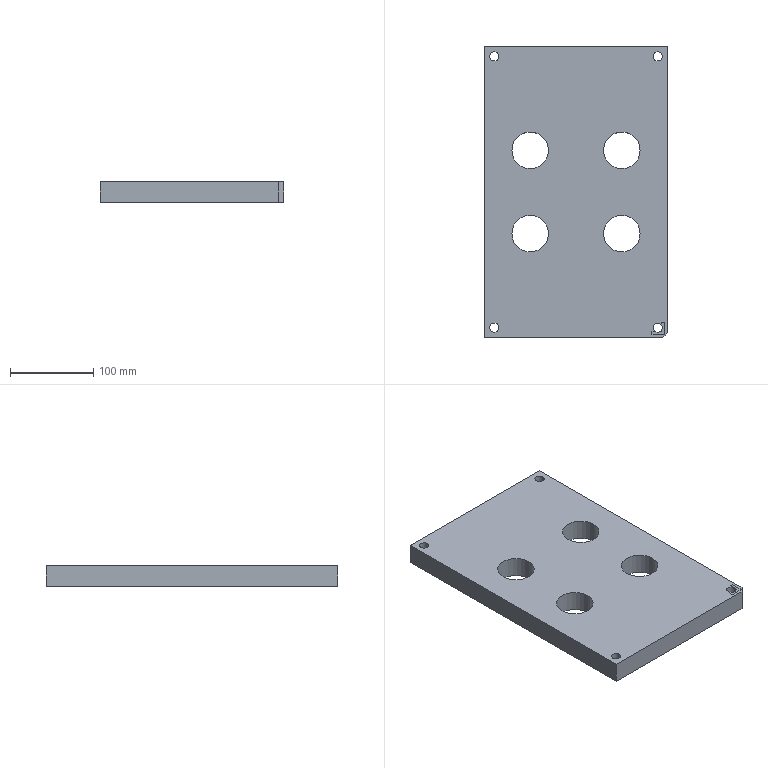Part | NX | features DZDB 2 | 1 solid | 33 faces | box 220 x 350 x 25 mm | volume 1756097 mm3 | plane 21 | cylinder 12 | commonest cylinder face diameters 11 x4 18 x4 44 x4
STEP:
#1=CARTESIAN_POINT('',(-77.,50.,-235.5));
#2=VERTEX_POINT('',#1);
#3=CARTESIAN_POINT('',(-55.,50.,-235.5));
#4=DIRECTION('',(0.,0.,-1.));
#5=DIRECTION('',(-1.,0.,0.));
#6=AXIS2_PLACEMENT_3D('',#3,#4,#5);
#7=CIRCLE('',#6,22.);
#8=EDGE_CURVE('',#2,#2,#7,.T.);
#9=ORIENTED_EDGE('',*,*,#8,.F.);
#10=EDGE_LOOP('',(#9));
#11=FACE_BOUND('',#10,.T.);
#12=CARTESIAN_POINT('',(33.,50.,-235.5));
#13=VERTEX_POINT('',#12);
#14=CARTESIAN_POINT('',(55.,50.,-235.5));
#15=DIRECTION('',(0.,0.,-1.));
#16=DIRECTION('',(-1.,0.,0.));
#17=AXIS2_PLACEMENT_3D('',#14,#15,#16);
#18=CIRCLE('',#17,22.);
#19=EDGE_CURVE('',#13,#13,#18,.T.);
#20=ORIENTED_EDGE('',*,*,#19,.F.);
#21=EDGE_LOOP('',(#20));
#22=FACE_BOUND('',#21,.T.);
#23=CARTESIAN_POINT('',(33.,-50.,-235.5));
#24=VERTEX_POINT('',#23);
#25=CARTESIAN_POINT('',(55.,-50.,-235.5));
#26=DIRECTION('',(0.,0.,-1.));
#27=DIRECTION('',(-1.,0.,0.));
#28=AXIS2_PLACEMENT_3D('',#25,#26,#27);
#29=CIRCLE('',#28,22.);
#30=EDGE_CURVE('',#24,#24,#29,.T.);
#31=ORIENTED_EDGE('',*,*,#30,.F.);
#32=EDGE_LOOP('',(#31));
#33=FACE_BOUND('',#32,.T.);
#34=CARTESIAN_POINT('',(-77.,-50.,-235.5));
#35=VERTEX_POINT('',#34);
#36=CARTESIAN_POINT('',(-55.,-50.,-235.5));
#37=DIRECTION('',(0.,0.,-1.));
#38=DIRECTION('',(-1.,0.,0.));
#39=AXIS2_PLACEMENT_3D('',#36,#37,#38);
#40=CIRCLE('',#39,22.);
#41=EDGE_CURVE('',#35,#35,#40,.T.);
#42=ORIENTED_EDGE('',*,*,#41,.F.);
#43=EDGE_LOOP('',(#42));
#44=FACE_BOUND('',#43,.T.);
#45=CARTESIAN_POINT('',(-107.,-163.,-235.5));
#46=VERTEX_POINT('',#45);
#47=CARTESIAN_POINT('',(-98.,-163.,-235.5));
#48=DIRECTION('',(0.,0.,1.));
#49=DIRECTION('',(-1.,0.,0.));
#50=AXIS2_PLACEMENT_3D('',#47,#48,#49);
#51=CIRCLE('',#50,9.);
#52=EDGE_CURVE('',#46,#46,#51,.T.);
#53=ORIENTED_EDGE('',*,*,#52,.T.);
#54=EDGE_LOOP('',(#53));
#55=FACE_BOUND('',#54,.T.);
#56=CARTESIAN_POINT('',(107.,163.,-235.5));
#57=VERTEX_POINT('',#56);
#58=CARTESIAN_POINT('',(98.,163.,-235.5));
#59=DIRECTION('',(0.,0.,1.));
#60=DIRECTION('',(1.,0.,0.));
#61=AXIS2_PLACEMENT_3D('',#58,#59,#60);
#62=CIRCLE('',#61,9.);
#63=EDGE_CURVE('',#57,#57,#62,.T.);
#64=ORIENTED_EDGE('',*,*,#63,.T.);
#65=EDGE_LOOP('',(#64));
#66=FACE_BOUND('',#65,.T.);
#67=CARTESIAN_POINT('',(110.,-169.,-235.5));
#68=VERTEX_POINT('',#67);
#69=CARTESIAN_POINT('',(110.,175.,-235.5));
#70=VERTEX_POINT('',#69);
#71=CARTESIAN_POINT('',(110.,0.,-235.5));
#72=DIRECTION('',(0.,1.,0.));
#73=VECTOR('',#72,1000.);
#74=LINE('',#71,#73);
#75=EDGE_CURVE('',#68,#70,#74,.T.);
#76=ORIENTED_EDGE('',*,*,#75,.F.);
#77=CARTESIAN_POINT('',(104.,-175.,-235.5));
#78=VERTEX_POINT('',#77);
#79=CARTESIAN_POINT('',(139.5,-139.5,-235.5));
#80=DIRECTION('',(0.7071,0.7071,0.));
#81=VECTOR('',#80,1000.);
#82=LINE('',#79,#81);
#83=EDGE_CURVE('',#68,#78,#82,.F.);
#84=ORIENTED_EDGE('',*,*,#83,.T.);
#85=CARTESIAN_POINT('',(-110.,-175.,-235.5));
#86=VERTEX_POINT('',#85);
#87=CARTESIAN_POINT('',(0.,-175.,-235.5));
#88=DIRECTION('',(1.,0.,0.));
#89=VECTOR('',#88,1000.);
#90=LINE('',#87,#89);
#91=EDGE_CURVE('',#86,#78,#90,.T.);
#92=ORIENTED_EDGE('',*,*,#91,.F.);
#93=CARTESIAN_POINT('',(-110.,175.,-235.5));
#94=VERTEX_POINT('',#93);
#95=CARTESIAN_POINT('',(-110.,0.,-235.5));
#96=DIRECTION('',(0.,-1.,0.));
#97=VECTOR('',#96,1000.);
#98=LINE('',#95,#97);
#99=EDGE_CURVE('',#94,#86,#98,.T.);
#100=ORIENTED_EDGE('',*,*,#99,.F.);
#101=CARTESIAN_POINT('',(0.,175.,-235.5));
#102=DIRECTION('',(-1.,0.,0.));
#103=VECTOR('',#102,1000.);
#104=LINE('',#101,#103);
#105=EDGE_CURVE('',#70,#94,#104,.T.);
#106=ORIENTED_EDGE('',*,*,#105,.F.);
#107=EDGE_LOOP('',(#76,#84,#92,#100,#106));
#108=FACE_BOUND('',#107,.T.);
#109=CARTESIAN_POINT('',(107.,-163.,-235.5));
#110=VERTEX_POINT('',#109);
#111=CARTESIAN_POINT('',(98.,-163.,-235.5));
#112=DIRECTION('',(0.,0.,1.));
#113=DIRECTION('',(1.,0.,0.));
#114=AXIS2_PLACEMENT_3D('',#111,#112,#113);
#115=CIRCLE('',#114,9.);
#116=EDGE_CURVE('',#110,#110,#115,.T.);
#117=ORIENTED_EDGE('',*,*,#116,.T.);
#118=EDGE_LOOP('',(#117));
#119=FACE_BOUND('',#118,.T.);
#120=CARTESIAN_POINT('',(-89.,163.,-235.5));
#121=VERTEX_POINT('',#120);
#122=CARTESIAN_POINT('',(-98.,163.,-235.5));
#123=DIRECTION('',(0.,0.,1.));
#124=DIRECTION('',(1.,0.,0.));
#125=AXIS2_PLACEMENT_3D('',#122,#123,#124);
#126=CIRCLE('',#125,9.);
#127=EDGE_CURVE('',#121,#121,#126,.T.);
#128=ORIENTED_EDGE('',*,*,#127,.T.);
#129=EDGE_LOOP('',(#128));
#130=FACE_BOUND('',#129,.T.);
#131=CARTESIAN_POINT('',(0.,0.,-235.5));
#132=DIRECTION('',(0.,0.,-1.));
#133=DIRECTION('',(-1.,0.,0.));
#134=AXIS2_PLACEMENT_3D('',#131,#132,#133);
#135=PLANE('',#134);
#136=ADVANCED_FACE('',(#11,#22,#33,#44,#55,#66,#108,#119,#130),#135,.T.);
#137=CARTESIAN_POINT('',(-33.,50.,-210.5));
#138=VERTEX_POINT('',#137);
#139=CARTESIAN_POINT('',(-55.,50.,-210.5));
#140=DIRECTION('',(0.,0.,1.));
#141=DIRECTION('',(1.,0.,0.));
#142=AXIS2_PLACEMENT_3D('',#139,#140,#141);
#143=CIRCLE('',#142,22.);
#144=EDGE_CURVE('',#138,#138,#143,.T.);
#145=ORIENTED_EDGE('',*,*,#144,.F.);
#146=EDGE_LOOP('',(#145));
#147=FACE_BOUND('',#146,.T.);
#148=CARTESIAN_POINT('',(77.,50.,-210.5));
#149=VERTEX_POINT('',#148);
#150=CARTESIAN_POINT('',(55.,50.,-210.5));
#151=DIRECTION('',(0.,0.,1.));
#152=DIRECTION('',(1.,0.,0.));
#153=AXIS2_PLACEMENT_3D('',#150,#151,#152);
#154=CIRCLE('',#153,22.);
#155=EDGE_CURVE('',#149,#149,#154,.T.);
#156=ORIENTED_EDGE('',*,*,#155,.F.);
#157=EDGE_LOOP('',(#156));
#158=FACE_BOUND('',#157,.T.);
#159=CARTESIAN_POINT('',(77.,-50.,-210.5));
#160=VERTEX_POINT('',#159);
#161=CARTESIAN_POINT('',(55.,-50.,-210.5));
#162=DIRECTION('',(0.,0.,1.));
#163=DIRECTION('',(1.,0.,0.));
#164=AXIS2_PLACEMENT_3D('',#161,#162,#163);
#165=CIRCLE('',#164,22.);
#166=EDGE_CURVE('',#160,#160,#165,.T.);
#167=ORIENTED_EDGE('',*,*,#166,.F.);
#168=EDGE_LOOP('',(#167));
#169=FACE_BOUND('',#168,.T.);
#170=CARTESIAN_POINT('',(-33.,-50.,-210.5));
#171=VERTEX_POINT('',#170);
#172=CARTESIAN_POINT('',(-55.,-50.,-210.5));
#173=DIRECTION('',(0.,0.,1.));
#174=DIRECTION('',(1.,0.,0.));
#175=AXIS2_PLACEMENT_3D('',#172,#173,#174);
#176=CIRCLE('',#175,22.);
#177=EDGE_CURVE('',#171,#171,#176,.T.);
#178=ORIENTED_EDGE('',*,*,#177,.F.);
#179=EDGE_LOOP('',(#178));
#180=FACE_BOUND('',#179,.T.);
#181=CARTESIAN_POINT('',(-103.5,-163.,-210.5));
#182=VERTEX_POINT('',#181);
#183=CARTESIAN_POINT('',(-98.,-163.,-210.5));
#184=DIRECTION('',(0.,0.,-1.));
#185=DIRECTION('',(-1.,0.,0.));
#186=AXIS2_PLACEMENT_3D('',#183,#184,#185);
#187=CIRCLE('',#186,5.5);
#188=EDGE_CURVE('',#182,#182,#187,.T.);
#189=ORIENTED_EDGE('',*,*,#188,.T.);
#190=EDGE_LOOP('',(#189));
#191=FACE_BOUND('',#190,.T.);
#192=CARTESIAN_POINT('',(103.5,163.,-210.5));
#193=VERTEX_POINT('',#192);
#194=CARTESIAN_POINT('',(98.,163.,-210.5));
#195=DIRECTION('',(0.,0.,-1.));
#196=DIRECTION('',(1.,0.,0.));
#197=AXIS2_PLACEMENT_3D('',#194,#195,#196);
#198=CIRCLE('',#197,5.5);
#199=EDGE_CURVE('',#193,#193,#198,.T.);
#200=ORIENTED_EDGE('',*,*,#199,.T.);
#201=EDGE_LOOP('',(#200));
#202=FACE_BOUND('',#201,.T.);
#203=CARTESIAN_POINT('',(104.,-175.,-210.5));
#204=VERTEX_POINT('',#203);
#205=CARTESIAN_POINT('',(-110.,-175.,-210.5));
#206=VERTEX_POINT('',#205);
#207=CARTESIAN_POINT('',(0.,-175.,-210.5));
#208=DIRECTION('',(-1.,0.,0.));
#209=VECTOR('',#208,1000.);
#210=LINE('',#207,#209);
#211=EDGE_CURVE('',#204,#206,#210,.T.);
#212=ORIENTED_EDGE('',*,*,#211,.F.);
#213=CARTESIAN_POINT('',(110.,-169.,-210.5));
#214=VERTEX_POINT('',#213);
#215=CARTESIAN_POINT('',(139.5,-139.5,-210.5));
#216=DIRECTION('',(-0.7071,-0.7071,0.));
#217=VECTOR('',#216,1000.);
#218=LINE('',#215,#217);
#219=EDGE_CURVE('',#204,#214,#218,.F.);
#220=ORIENTED_EDGE('',*,*,#219,.T.);
#221=CARTESIAN_POINT('',(110.,175.,-210.5));
#222=VERTEX_POINT('',#221);
#223=CARTESIAN_POINT('',(110.,0.,-210.5));
#224=DIRECTION('',(0.,-1.,0.));
#225=VECTOR('',#224,1000.);
#226=LINE('',#223,#225);
#227=EDGE_CURVE('',#222,#214,#226,.T.);
#228=ORIENTED_EDGE('',*,*,#227,.F.);
#229=CARTESIAN_POINT('',(-110.,175.,-210.5));
#230=VERTEX_POINT('',#229);
#231=CARTESIAN_POINT('',(0.,175.,-210.5));
#232=DIRECTION('',(1.,0.,0.));
#233=VECTOR('',#232,1000.);
#234=LINE('',#231,#233);
#235=EDGE_CURVE('',#230,#222,#234,.T.);
#236=ORIENTED_EDGE('',*,*,#235,.F.);
#237=CARTESIAN_POINT('',(-110.,0.,-210.5));
#238=DIRECTION('',(0.,1.,0.));
#239=VECTOR('',#238,1000.);
#240=LINE('',#237,#239);
#241=EDGE_CURVE('',#206,#230,#240,.T.);
#242=ORIENTED_EDGE('',*,*,#241,.F.);
#243=EDGE_LOOP('',(#212,#220,#228,#236,#242));
#244=FACE_BOUND('',#243,.T.);
#245=CARTESIAN_POINT('',(94.838,-167.5,-210.5));
#246=VERTEX_POINT('',#245);
#247=CARTESIAN_POINT('',(91.25,-167.5,-210.5));
#248=VERTEX_POINT('',#247);
#249=CARTESIAN_POINT('',(96.875,-167.5,-210.5));
#250=DIRECTION('',(-1.,0.,0.));
#251=VECTOR('',#250,1000.);
#252=LINE('',#249,#251);
#253=EDGE_CURVE('',#246,#248,#252,.T.);
#254=ORIENTED_EDGE('',*,*,#253,.F.);
#255=CARTESIAN_POINT('',(102.5,-159.838,-210.5));
#256=VERTEX_POINT('',#255);
#257=CARTESIAN_POINT('',(98.,-163.,-210.5));
#258=DIRECTION('',(0.,0.,-1.));
#259=DIRECTION('',(1.,0.,0.));
#260=AXIS2_PLACEMENT_3D('',#257,#258,#259);
#261=CIRCLE('',#260,5.5);
#262=EDGE_CURVE('',#246,#256,#261,.T.);
#263=ORIENTED_EDGE('',*,*,#262,.T.);
#264=CARTESIAN_POINT('',(102.5,-156.25,-210.5));
#265=VERTEX_POINT('',#264);
#266=CARTESIAN_POINT('',(102.5,-161.875,-210.5));
#267=DIRECTION('',(0.,-1.,0.));
#268=VECTOR('',#267,1000.);
#269=LINE('',#266,#268);
#270=EDGE_CURVE('',#265,#256,#269,.T.);
#271=ORIENTED_EDGE('',*,*,#270,.F.);
#272=CARTESIAN_POINT('',(106.25,-156.25,-210.5));
#273=VERTEX_POINT('',#272);
#274=CARTESIAN_POINT('',(98.75,-156.25,-210.5));
#275=DIRECTION('',(1.,0.,0.));
#276=VECTOR('',#275,1000.);
#277=LINE('',#274,#276);
#278=EDGE_CURVE('',#265,#273,#277,.T.);
#279=ORIENTED_EDGE('',*,*,#278,.T.);
#280=CARTESIAN_POINT('',(106.25,-171.25,-210.5));
#281=VERTEX_POINT('',#280);
#282=CARTESIAN_POINT('',(106.25,-163.75,-210.5));
#283=DIRECTION('',(0.,-1.,0.));
#284=VECTOR('',#283,1000.);
#285=LINE('',#282,#284);
#286=EDGE_CURVE('',#273,#281,#285,.T.);
#287=ORIENTED_EDGE('',*,*,#286,.T.);
#288=CARTESIAN_POINT('',(91.25,-171.25,-210.5));
#289=VERTEX_POINT('',#288);
#290=CARTESIAN_POINT('',(98.75,-171.25,-210.5));
#291=DIRECTION('',(-1.,0.,0.));
#292=VECTOR('',#291,1000.);
#293=LINE('',#290,#292);
#294=EDGE_CURVE('',#281,#289,#293,.T.);
#295=ORIENTED_EDGE('',*,*,#294,.T.);
#296=CARTESIAN_POINT('',(91.25,-163.75,-210.5));
#297=DIRECTION('',(0.,1.,0.));
#298=VECTOR('',#297,1000.);
#299=LINE('',#296,#298);
#300=EDGE_CURVE('',#289,#248,#299,.T.);
#301=ORIENTED_EDGE('',*,*,#300,.T.);
#302=EDGE_LOOP('',(#254,#263,#271,#279,#287,#295,#301));
#303=FACE_BOUND('',#302,.T.);
#304=CARTESIAN_POINT('',(-92.5,163.,-210.5));
#305=VERTEX_POINT('',#304);
#306=CARTESIAN_POINT('',(-98.,163.,-210.5));
#307=DIRECTION('',(0.,0.,-1.));
#308=DIRECTION('',(1.,0.,0.));
#309=AXIS2_PLACEMENT_3D('',#306,#307,#308);
#310=CIRCLE('',#309,5.5);
#311=EDGE_CURVE('',#305,#305,#310,.T.);
#312=ORIENTED_EDGE('',*,*,#311,.T.);
#313=EDGE_LOOP('',(#312));
#314=FACE_BOUND('',#313,.T.);
#315=CARTESIAN_POINT('',(0.,0.,-210.5));
#316=DIRECTION('',(0.,0.,1.));
#317=DIRECTION('',(1.,0.,0.));
#318=AXIS2_PLACEMENT_3D('',#315,#316,#317);
#319=PLANE('',#318);
#320=ADVANCED_FACE('',(#147,#158,#169,#180,#191,#202,#244,#303,#314),#319,.T.);
#321=CARTESIAN_POINT('',(102.5,-166.162,-210.5));
#322=VERTEX_POINT('',#321);
#323=CARTESIAN_POINT('',(102.5,-167.5,-210.5));
#324=VERTEX_POINT('',#323);
#325=CARTESIAN_POINT('',(102.5,-161.875,-210.5));
#326=DIRECTION('',(0.,-1.,0.));
#327=VECTOR('',#326,1000.);
#328=LINE('',#325,#327);
#329=EDGE_CURVE('',#322,#324,#328,.T.);
#330=ORIENTED_EDGE('',*,*,#329,.F.);
#331=CARTESIAN_POINT('',(101.162,-167.5,-210.5));
#332=VERTEX_POINT('',#331);
#333=CARTESIAN_POINT('',(98.,-163.,-210.5));
#334=DIRECTION('',(0.,0.,-1.));
#335=DIRECTION('',(1.,0.,0.));
#336=AXIS2_PLACEMENT_3D('',#333,#334,#335);
#337=CIRCLE('',#336,5.5);
#338=EDGE_CURVE('',#322,#332,#337,.T.);
#339=ORIENTED_EDGE('',*,*,#338,.T.);
#340=CARTESIAN_POINT('',(96.875,-167.5,-210.5));
#341=DIRECTION('',(-1.,0.,0.));
#342=VECTOR('',#341,1000.);
#343=LINE('',#340,#342);
#344=EDGE_CURVE('',#324,#332,#343,.T.);
#345=ORIENTED_EDGE('',*,*,#344,.F.);
#346=EDGE_LOOP('',(#330,#339,#345));
#347=FACE_BOUND('',#346,.T.);
#348=CARTESIAN_POINT('',(0.,0.,-210.5));
#349=DIRECTION('',(0.,0.,1.));
#350=DIRECTION('',(1.,0.,0.));
#351=AXIS2_PLACEMENT_3D('',#348,#349,#350);
#352=PLANE('',#351);
#353=ADVANCED_FACE('',(#347),#352,.T.);
#354=CARTESIAN_POINT('',(101.162,-167.5,-210.6));
#355=VERTEX_POINT('',#354);
#356=CARTESIAN_POINT('',(101.162,-167.5,-235.5));
#357=DIRECTION('',(0.,0.,1.));
#358=VECTOR('',#357,1000.);
#359=LINE('',#356,#358);
#360=EDGE_CURVE('',#355,#332,#359,.T.);
#361=ORIENTED_EDGE('',*,*,#360,.F.);
#362=CARTESIAN_POINT('',(102.5,-167.5,-210.6));
#363=VERTEX_POINT('',#362);
#364=CARTESIAN_POINT('',(96.875,-167.5,-210.6));
#365=DIRECTION('',(1.,0.,0.));
#366=VECTOR('',#365,1000.);
#367=LINE('',#364,#366);
#368=EDGE_CURVE('',#363,#355,#367,.F.);
#369=ORIENTED_EDGE('',*,*,#368,.F.);
#370=CARTESIAN_POINT('',(102.5,-167.5,-210.6));
#371=DIRECTION('',(0.,0.,1.));
#372=VECTOR('',#371,1000.);
#373=LINE('',#370,#372);
#374=EDGE_CURVE('',#363,#324,#373,.T.);
#375=ORIENTED_EDGE('',*,*,#374,.T.);
#376=ORIENTED_EDGE('',*,*,#344,.T.);
#377=EDGE_LOOP('',(#361,#369,#375,#376));
#378=FACE_BOUND('',#377,.T.);
#379=CARTESIAN_POINT('',(96.875,-167.5,-210.6));
#380=DIRECTION('',(0.,-1.,0.));
#381=DIRECTION('',(0.,0.,-1.));
#382=AXIS2_PLACEMENT_3D('',#379,#380,#381);
#383=PLANE('',#382);
#384=ADVANCED_FACE('',(#378),#383,.T.);
#385=CARTESIAN_POINT('',(102.5,-159.838,-210.6));
#386=VERTEX_POINT('',#385);
#387=CARTESIAN_POINT('',(102.5,-159.838,-235.5));
#388=DIRECTION('',(0.,0.,1.));
#389=VECTOR('',#388,1000.);
#390=LINE('',#387,#389);
#391=EDGE_CURVE('',#386,#256,#390,.T.);
#392=ORIENTED_EDGE('',*,*,#391,.F.);
#393=CARTESIAN_POINT('',(102.5,-156.25,-210.6));
#394=VERTEX_POINT('',#393);
#395=CARTESIAN_POINT('',(102.5,-161.875,-210.6));
#396=DIRECTION('',(0.,1.,0.));
#397=VECTOR('',#396,1000.);
#398=LINE('',#395,#397);
#399=EDGE_CURVE('',#394,#386,#398,.F.);
#400=ORIENTED_EDGE('',*,*,#399,.F.);
#401=CARTESIAN_POINT('',(102.5,-156.25,-210.6));
#402=DIRECTION('',(0.,0.,1.));
#403=VECTOR('',#402,1000.);
#404=LINE('',#401,#403);
#405=EDGE_CURVE('',#265,#394,#404,.F.);
#406=ORIENTED_EDGE('',*,*,#405,.F.);
#407=ORIENTED_EDGE('',*,*,#270,.T.);
#408=EDGE_LOOP('',(#392,#400,#406,#407));
#409=FACE_BOUND('',#408,.T.);
#410=CARTESIAN_POINT('',(102.5,-161.875,-210.6));
#411=DIRECTION('',(1.,0.,0.));
#412=DIRECTION('',(0.,0.,-1.));
#413=AXIS2_PLACEMENT_3D('',#410,#411,#412);
#414=PLANE('',#413);
#415=ADVANCED_FACE('',(#409),#414,.T.);
#416=ORIENTED_EDGE('',*,*,#91,.T.);
#417=CARTESIAN_POINT('',(104.,-175.,-235.5));
#418=DIRECTION('',(0.,0.,1.));
#419=VECTOR('',#418,1000.);
#420=LINE('',#417,#419);
#421=EDGE_CURVE('',#78,#204,#420,.T.);
#422=ORIENTED_EDGE('',*,*,#421,.T.);
#423=ORIENTED_EDGE('',*,*,#211,.T.);
#424=CARTESIAN_POINT('',(-110.,-175.,-235.5));
#425=DIRECTION('',(0.,0.,1.));
#426=VECTOR('',#425,1000.);
#427=LINE('',#424,#426);
#428=EDGE_CURVE('',#86,#206,#427,.T.);
#429=ORIENTED_EDGE('',*,*,#428,.F.);
#430=EDGE_LOOP('',(#416,#422,#423,#429));
#431=FACE_BOUND('',#430,.T.);
#432=CARTESIAN_POINT('',(0.,-175.,-235.5));
#433=DIRECTION('',(0.,-1.,0.));
#434=DIRECTION('',(0.,0.,-1.));
#435=AXIS2_PLACEMENT_3D('',#432,#433,#434);
#436=PLANE('',#435);
#437=ADVANCED_FACE('',(#431),#436,.T.);
#438=ORIENTED_EDGE('',*,*,#428,.T.);
#439=ORIENTED_EDGE('',*,*,#241,.T.);
#440=CARTESIAN_POINT('',(-110.,175.,-235.5));
#441=DIRECTION('',(0.,0.,1.));
#442=VECTOR('',#441,1000.);
#443=LINE('',#440,#442);
#444=EDGE_CURVE('',#94,#230,#443,.T.);
#445=ORIENTED_EDGE('',*,*,#444,.F.);
#446=ORIENTED_EDGE('',*,*,#99,.T.);
#447=EDGE_LOOP('',(#438,#439,#445,#446));
#448=FACE_BOUND('',#447,.T.);
#449=CARTESIAN_POINT('',(-110.,0.,-235.5));
#450=DIRECTION('',(-1.,0.,0.));
#451=DIRECTION('',(0.,0.,1.));
#452=AXIS2_PLACEMENT_3D('',#449,#450,#451);
#453=PLANE('',#452);
#454=ADVANCED_FACE('',(#448),#453,.T.);
#455=ORIENTED_EDGE('',*,*,#444,.T.);
#456=ORIENTED_EDGE('',*,*,#235,.T.);
#457=CARTESIAN_POINT('',(110.,175.,-235.5));
#458=DIRECTION('',(0.,0.,1.));
#459=VECTOR('',#458,1000.);
#460=LINE('',#457,#459);
#461=EDGE_CURVE('',#70,#222,#460,.T.);
#462=ORIENTED_EDGE('',*,*,#461,.F.);
#463=ORIENTED_EDGE('',*,*,#105,.T.);
#464=EDGE_LOOP('',(#455,#456,#462,#463));
#465=FACE_BOUND('',#464,.T.);
#466=CARTESIAN_POINT('',(0.,175.,-235.5));
#467=DIRECTION('',(0.,1.,0.));
#468=DIRECTION('',(0.,0.,1.));
#469=AXIS2_PLACEMENT_3D('',#466,#467,#468);
#470=PLANE('',#469);
#471=ADVANCED_FACE('',(#465),#470,.T.);
#472=ORIENTED_EDGE('',*,*,#227,.T.);
#473=CARTESIAN_POINT('',(110.,-169.,-235.5));
#474=DIRECTION('',(0.,0.,-1.));
#475=VECTOR('',#474,1000.);
#476=LINE('',#473,#475);
#477=EDGE_CURVE('',#214,#68,#476,.T.);
#478=ORIENTED_EDGE('',*,*,#477,.T.);
#479=ORIENTED_EDGE('',*,*,#75,.T.);
#480=ORIENTED_EDGE('',*,*,#461,.T.);
#481=EDGE_LOOP('',(#472,#478,#479,#480));
#482=FACE_BOUND('',#481,.T.);
#483=CARTESIAN_POINT('',(110.,0.,-235.5));
#484=DIRECTION('',(1.,0.,0.));
#485=DIRECTION('',(0.,0.,-1.));
#486=AXIS2_PLACEMENT_3D('',#483,#484,#485);
#487=PLANE('',#486);
#488=ADVANCED_FACE('',(#482),#487,.T.);
#489=CARTESIAN_POINT('',(106.25,-156.25,-210.6));
#490=VERTEX_POINT('',#489);
#491=CARTESIAN_POINT('',(98.75,-156.25,-210.6));
#492=DIRECTION('',(-1.,0.,0.));
#493=VECTOR('',#492,1000.);
#494=LINE('',#491,#493);
#495=EDGE_CURVE('',#394,#490,#494,.F.);
#496=ORIENTED_EDGE('',*,*,#495,.T.);
#497=CARTESIAN_POINT('',(106.25,-156.25,-210.6));
#498=DIRECTION('',(0.,0.,1.));
#499=VECTOR('',#498,1000.);
#500=LINE('',#497,#499);
#501=EDGE_CURVE('',#273,#490,#500,.F.);
#502=ORIENTED_EDGE('',*,*,#501,.F.);
#503=ORIENTED_EDGE('',*,*,#278,.F.);
#504=ORIENTED_EDGE('',*,*,#405,.T.);
#505=EDGE_LOOP('',(#496,#502,#503,#504));
#506=FACE_BOUND('',#505,.T.);
#507=CARTESIAN_POINT('',(98.75,-156.25,-210.6));
#508=DIRECTION('',(0.,1.,0.));
#509=DIRECTION('',(0.,0.,1.));
#510=AXIS2_PLACEMENT_3D('',#507,#508,#509);
#511=PLANE('',#510);
#512=ADVANCED_FACE('',(#506),#511,.F.);
#513=ORIENTED_EDGE('',*,*,#399,.T.);
#514=CARTESIAN_POINT('',(102.5,-166.162,-210.6));
#515=VERTEX_POINT('',#514);
#516=CARTESIAN_POINT('',(98.,-163.,-210.6));
#517=DIRECTION('',(0.,0.,-1.));
#518=DIRECTION('',(-1.,0.,0.));
#519=AXIS2_PLACEMENT_3D('',#516,#517,#518);
#520=CIRCLE('',#519,5.5);
#521=EDGE_CURVE('',#386,#515,#520,.T.);
#522=ORIENTED_EDGE('',*,*,#521,.T.);
#523=CARTESIAN_POINT('',(102.5,-161.875,-210.6));
#524=DIRECTION('',(0.,1.,0.));
#525=VECTOR('',#524,1000.);
#526=LINE('',#523,#525);
#527=EDGE_CURVE('',#515,#363,#526,.F.);
#528=ORIENTED_EDGE('',*,*,#527,.T.);
#529=ORIENTED_EDGE('',*,*,#368,.T.);
#530=CARTESIAN_POINT('',(94.838,-167.5,-210.6));
#531=VERTEX_POINT('',#530);
#532=CARTESIAN_POINT('',(98.,-163.,-210.6));
#533=DIRECTION('',(0.,0.,-1.));
#534=DIRECTION('',(-1.,0.,0.));
#535=AXIS2_PLACEMENT_3D('',#532,#533,#534);
#536=CIRCLE('',#535,5.5);
#537=EDGE_CURVE('',#355,#531,#536,.T.);
#538=ORIENTED_EDGE('',*,*,#537,.T.);
#539=CARTESIAN_POINT('',(91.25,-167.5,-210.6));
#540=VERTEX_POINT('',#539);
#541=CARTESIAN_POINT('',(96.875,-167.5,-210.6));
#542=DIRECTION('',(1.,0.,0.));
#543=VECTOR('',#542,1000.);
#544=LINE('',#541,#543);
#545=EDGE_CURVE('',#531,#540,#544,.F.);
#546=ORIENTED_EDGE('',*,*,#545,.T.);
#547=CARTESIAN_POINT('',(91.25,-171.25,-210.6));
#548=VERTEX_POINT('',#547);
#549=CARTESIAN_POINT('',(91.25,-163.75,-210.6));
#550=DIRECTION('',(0.,-1.,0.));
#551=VECTOR('',#550,1000.);
#552=LINE('',#549,#551);
#553=EDGE_CURVE('',#548,#540,#552,.F.);
#554=ORIENTED_EDGE('',*,*,#553,.F.);
#555=CARTESIAN_POINT('',(106.25,-171.25,-210.6));
#556=VERTEX_POINT('',#555);
#557=CARTESIAN_POINT('',(98.75,-171.25,-210.6));
#558=DIRECTION('',(1.,0.,0.));
#559=VECTOR('',#558,1000.);
#560=LINE('',#557,#559);
#561=EDGE_CURVE('',#556,#548,#560,.F.);
#562=ORIENTED_EDGE('',*,*,#561,.F.);
#563=CARTESIAN_POINT('',(106.25,-163.75,-210.6));
#564=DIRECTION('',(0.,1.,0.));
#565=VECTOR('',#564,1000.);
#566=LINE('',#563,#565);
#567=EDGE_CURVE('',#490,#556,#566,.F.);
#568=ORIENTED_EDGE('',*,*,#567,.F.);
#569=ORIENTED_EDGE('',*,*,#495,.F.);
#570=EDGE_LOOP('',(#513,#522,#528,#529,#538,#546,#554,#562,#568,#569));
#571=FACE_BOUND('',#570,.T.);
#572=CARTESIAN_POINT('',(98.75,-163.75,-210.6));
#573=DIRECTION('',(0.,0.,-1.));
#574=DIRECTION('',(-1.,0.,0.));
#575=AXIS2_PLACEMENT_3D('',#572,#573,#574);
#576=PLANE('',#575);
#577=ADVANCED_FACE('',(#571),#576,.F.);
#578=CARTESIAN_POINT('',(106.25,-171.25,-210.6));
#579=DIRECTION('',(0.,0.,1.));
#580=VECTOR('',#579,1000.);
#581=LINE('',#578,#580);
#582=EDGE_CURVE('',#281,#556,#581,.F.);
#583=ORIENTED_EDGE('',*,*,#582,.T.);
#584=ORIENTED_EDGE('',*,*,#561,.T.);
#585=CARTESIAN_POINT('',(91.25,-171.25,-210.6));
#586=DIRECTION('',(0.,0.,1.));
#587=VECTOR('',#586,1000.);
#588=LINE('',#585,#587);
#589=EDGE_CURVE('',#289,#548,#588,.F.);
#590=ORIENTED_EDGE('',*,*,#589,.F.);
#591=ORIENTED_EDGE('',*,*,#294,.F.);
#592=EDGE_LOOP('',(#583,#584,#590,#591));
#593=FACE_BOUND('',#592,.T.);
#594=CARTESIAN_POINT('',(98.75,-171.25,-210.6));
#595=DIRECTION('',(0.,-1.,0.));
#596=DIRECTION('',(0.,0.,-1.));
#597=AXIS2_PLACEMENT_3D('',#594,#595,#596);
#598=PLANE('',#597);
#599=ADVANCED_FACE('',(#593),#598,.F.);
#600=CARTESIAN_POINT('',(91.25,-167.5,-210.6));
#601=DIRECTION('',(0.,0.,1.));
#602=VECTOR('',#601,1000.);
#603=LINE('',#600,#602);
#604=EDGE_CURVE('',#248,#540,#603,.F.);
#605=ORIENTED_EDGE('',*,*,#604,.F.);
#606=ORIENTED_EDGE('',*,*,#300,.F.);
#607=ORIENTED_EDGE('',*,*,#589,.T.);
#608=ORIENTED_EDGE('',*,*,#553,.T.);
#609=EDGE_LOOP('',(#605,#606,#607,#608));
#610=FACE_BOUND('',#609,.T.);
#611=CARTESIAN_POINT('',(91.25,-163.75,-210.6));
#612=DIRECTION('',(-1.,0.,0.));
#613=DIRECTION('',(0.,0.,1.));
#614=AXIS2_PLACEMENT_3D('',#611,#612,#613);
#615=PLANE('',#614);
#616=ADVANCED_FACE('',(#610),#615,.F.);
#617=ORIENTED_EDGE('',*,*,#567,.T.);
#618=ORIENTED_EDGE('',*,*,#582,.F.);
#619=ORIENTED_EDGE('',*,*,#286,.F.);
#620=ORIENTED_EDGE('',*,*,#501,.T.);
#621=EDGE_LOOP('',(#617,#618,#619,#620));
#622=FACE_BOUND('',#621,.T.);
#623=CARTESIAN_POINT('',(106.25,-163.75,-210.6));
#624=DIRECTION('',(1.,0.,0.));
#625=DIRECTION('',(0.,0.,-1.));
#626=AXIS2_PLACEMENT_3D('',#623,#624,#625);
#627=PLANE('',#626);
#628=ADVANCED_FACE('',(#622),#627,.F.);
#629=CARTESIAN_POINT('',(94.838,-167.5,-235.5));
#630=DIRECTION('',(0.,0.,1.));
#631=VECTOR('',#630,1000.);
#632=LINE('',#629,#631);
#633=EDGE_CURVE('',#246,#531,#632,.F.);
#634=ORIENTED_EDGE('',*,*,#633,.F.);
#635=ORIENTED_EDGE('',*,*,#253,.T.);
#636=ORIENTED_EDGE('',*,*,#604,.T.);
#637=ORIENTED_EDGE('',*,*,#545,.F.);
#638=EDGE_LOOP('',(#634,#635,#636,#637));
#639=FACE_BOUND('',#638,.T.);
#640=CARTESIAN_POINT('',(96.875,-167.5,-210.6));
#641=DIRECTION('',(0.,-1.,0.));
#642=DIRECTION('',(0.,0.,-1.));
#643=AXIS2_PLACEMENT_3D('',#640,#641,#642);
#644=PLANE('',#643);
#645=ADVANCED_FACE('',(#639),#644,.T.);
#646=CARTESIAN_POINT('',(102.5,-166.162,-235.5));
#647=DIRECTION('',(0.,0.,1.));
#648=VECTOR('',#647,1000.);
#649=LINE('',#646,#648);
#650=EDGE_CURVE('',#322,#515,#649,.F.);
#651=ORIENTED_EDGE('',*,*,#650,.F.);
#652=ORIENTED_EDGE('',*,*,#329,.T.);
#653=ORIENTED_EDGE('',*,*,#374,.F.);
#654=ORIENTED_EDGE('',*,*,#527,.F.);
#655=EDGE_LOOP('',(#651,#652,#653,#654));
#656=FACE_BOUND('',#655,.T.);
#657=CARTESIAN_POINT('',(102.5,-161.875,-210.6));
#658=DIRECTION('',(1.,0.,0.));
#659=DIRECTION('',(0.,0.,-1.));
#660=AXIS2_PLACEMENT_3D('',#657,#658,#659);
#661=PLANE('',#660);
#662=ADVANCED_FACE('',(#656),#661,.T.);
#663=CARTESIAN_POINT('',(103.5,163.,-224.7));
#664=VERTEX_POINT('',#663);
#665=CARTESIAN_POINT('',(98.,163.,-224.7));
#666=DIRECTION('',(0.,0.,1.));
#667=DIRECTION('',(1.,0.,0.));
#668=AXIS2_PLACEMENT_3D('',#665,#666,#667);
#669=CIRCLE('',#668,5.5);
#670=EDGE_CURVE('',#664,#664,#669,.T.);
#671=ORIENTED_EDGE('',*,*,#670,.F.);
#672=EDGE_LOOP('',(#671));
#673=FACE_BOUND('',#672,.T.);
#674=ORIENTED_EDGE('',*,*,#199,.F.);
#675=EDGE_LOOP('',(#674));
#676=FACE_BOUND('',#675,.T.);
#677=CARTESIAN_POINT('',(98.,163.,-235.5));
#678=DIRECTION('',(0.,0.,1.));
#679=DIRECTION('',(1.,0.,0.));
#680=AXIS2_PLACEMENT_3D('',#677,#678,#679);
#681=CYLINDRICAL_SURFACE('',#680,5.5);
#682=ADVANCED_FACE('',(#673,#676),#681,.F.);
#683=ORIENTED_EDGE('',*,*,#670,.T.);
#684=EDGE_LOOP('',(#683));
#685=FACE_BOUND('',#684,.T.);
#686=CARTESIAN_POINT('',(107.,163.,-224.7));
#687=VERTEX_POINT('',#686);
#688=CARTESIAN_POINT('',(98.,163.,-224.7));
#689=DIRECTION('',(0.,0.,-1.));
#690=DIRECTION('',(1.,0.,0.));
#691=AXIS2_PLACEMENT_3D('',#688,#689,#690);
#692=CIRCLE('',#691,9.);
#693=EDGE_CURVE('',#687,#687,#692,.F.);
#694=ORIENTED_EDGE('',*,*,#693,.F.);
#695=EDGE_LOOP('',(#694));
#696=FACE_BOUND('',#695,.T.);
#697=CARTESIAN_POINT('',(98.,163.,-224.7));
#698=DIRECTION('',(0.,0.,1.));
#699=DIRECTION('',(1.,0.,0.));
#700=AXIS2_PLACEMENT_3D('',#697,#698,#699);
#701=PLANE('',#700);
#702=ADVANCED_FACE('',(#685,#696),#701,.F.);
#703=ORIENTED_EDGE('',*,*,#693,.T.);
#704=EDGE_LOOP('',(#703));
#705=FACE_BOUND('',#704,.T.);
#706=ORIENTED_EDGE('',*,*,#63,.F.);
#707=EDGE_LOOP('',(#706));
#708=FACE_BOUND('',#707,.T.);
#709=CARTESIAN_POINT('',(98.,163.,-235.5));
#710=DIRECTION('',(0.,0.,1.));
#711=DIRECTION('',(1.,0.,0.));
#712=AXIS2_PLACEMENT_3D('',#709,#710,#711);
#713=CYLINDRICAL_SURFACE('',#712,9.);
#714=ADVANCED_FACE('',(#705,#708),#713,.F.);
#715=ORIENTED_EDGE('',*,*,#360,.T.);
#716=ORIENTED_EDGE('',*,*,#338,.F.);
#717=ORIENTED_EDGE('',*,*,#650,.T.);
#718=ORIENTED_EDGE('',*,*,#521,.F.);
#719=ORIENTED_EDGE('',*,*,#391,.T.);
#720=ORIENTED_EDGE('',*,*,#262,.F.);
#721=ORIENTED_EDGE('',*,*,#633,.T.);
#722=ORIENTED_EDGE('',*,*,#537,.F.);
#723=EDGE_LOOP('',(#715,#716,#717,#718,#719,#720,#721,#722));
#724=FACE_BOUND('',#723,.T.);
#725=CARTESIAN_POINT('',(103.5,-163.,-224.7));
#726=VERTEX_POINT('',#725);
#727=CARTESIAN_POINT('',(98.,-163.,-224.7));
#728=DIRECTION('',(0.,0.,1.));
#729=DIRECTION('',(1.,0.,0.));
#730=AXIS2_PLACEMENT_3D('',#727,#728,#729);
#731=CIRCLE('',#730,5.5);
#732=EDGE_CURVE('',#726,#726,#731,.T.);
#733=ORIENTED_EDGE('',*,*,#732,.F.);
#734=EDGE_LOOP('',(#733));
#735=FACE_BOUND('',#734,.T.);
#736=CARTESIAN_POINT('',(98.,-163.,-235.5));
#737=DIRECTION('',(0.,0.,1.));
#738=DIRECTION('',(1.,0.,0.));
#739=AXIS2_PLACEMENT_3D('',#736,#737,#738);
#740=CYLINDRICAL_SURFACE('',#739,5.5);
#741=ADVANCED_FACE('',(#724,#735),#740,.F.);
#742=ORIENTED_EDGE('',*,*,#732,.T.);
#743=EDGE_LOOP('',(#742));
#744=FACE_BOUND('',#743,.T.);
#745=CARTESIAN_POINT('',(107.,-163.,-224.7));
#746=VERTEX_POINT('',#745);
#747=CARTESIAN_POINT('',(98.,-163.,-224.7));
#748=DIRECTION('',(0.,0.,-1.));
#749=DIRECTION('',(1.,0.,0.));
#750=AXIS2_PLACEMENT_3D('',#747,#748,#749);
#751=CIRCLE('',#750,9.);
#752=EDGE_CURVE('',#746,#746,#751,.F.);
#753=ORIENTED_EDGE('',*,*,#752,.F.);
#754=EDGE_LOOP('',(#753));
#755=FACE_BOUND('',#754,.T.);
#756=CARTESIAN_POINT('',(98.,-163.,-224.7));
#757=DIRECTION('',(0.,0.,1.));
#758=DIRECTION('',(1.,0.,0.));
#759=AXIS2_PLACEMENT_3D('',#756,#757,#758);
#760=PLANE('',#759);
#761=ADVANCED_FACE('',(#744,#755),#760,.F.);
#762=ORIENTED_EDGE('',*,*,#752,.T.);
#763=EDGE_LOOP('',(#762));
#764=FACE_BOUND('',#763,.T.);
#765=ORIENTED_EDGE('',*,*,#116,.F.);
#766=EDGE_LOOP('',(#765));
#767=FACE_BOUND('',#766,.T.);
#768=CARTESIAN_POINT('',(98.,-163.,-235.5));
#769=DIRECTION('',(0.,0.,1.));
#770=DIRECTION('',(1.,0.,0.));
#771=AXIS2_PLACEMENT_3D('',#768,#769,#770);
#772=CYLINDRICAL_SURFACE('',#771,9.);
#773=ADVANCED_FACE('',(#764,#767),#772,.F.);
#774=CARTESIAN_POINT('',(-103.5,-163.,-224.7));
#775=VERTEX_POINT('',#774);
#776=CARTESIAN_POINT('',(-98.,-163.,-224.7));
#777=DIRECTION('',(0.,0.,1.));
#778=DIRECTION('',(-1.,0.,0.));
#779=AXIS2_PLACEMENT_3D('',#776,#777,#778);
#780=CIRCLE('',#779,5.5);
#781=EDGE_CURVE('',#775,#775,#780,.T.);
#782=ORIENTED_EDGE('',*,*,#781,.F.);
#783=EDGE_LOOP('',(#782));
#784=FACE_BOUND('',#783,.T.);
#785=ORIENTED_EDGE('',*,*,#188,.F.);
#786=EDGE_LOOP('',(#785));
#787=FACE_BOUND('',#786,.T.);
#788=CARTESIAN_POINT('',(-98.,-163.,-235.5));
#789=DIRECTION('',(0.,0.,1.));
#790=DIRECTION('',(-1.,0.,0.));
#791=AXIS2_PLACEMENT_3D('',#788,#789,#790);
#792=CYLINDRICAL_SURFACE('',#791,5.5);
#793=ADVANCED_FACE('',(#784,#787),#792,.F.);
#794=ORIENTED_EDGE('',*,*,#781,.T.);
#795=EDGE_LOOP('',(#794));
#796=FACE_BOUND('',#795,.T.);
#797=CARTESIAN_POINT('',(-107.,-163.,-224.7));
#798=VERTEX_POINT('',#797);
#799=CARTESIAN_POINT('',(-98.,-163.,-224.7));
#800=DIRECTION('',(0.,0.,-1.));
#801=DIRECTION('',(-1.,0.,0.));
#802=AXIS2_PLACEMENT_3D('',#799,#800,#801);
#803=CIRCLE('',#802,9.);
#804=EDGE_CURVE('',#798,#798,#803,.F.);
#805=ORIENTED_EDGE('',*,*,#804,.F.);
#806=EDGE_LOOP('',(#805));
#807=FACE_BOUND('',#806,.T.);
#808=CARTESIAN_POINT('',(-98.,-163.,-224.7));
#809=DIRECTION('',(0.,0.,1.));
#810=DIRECTION('',(-1.,0.,0.));
#811=AXIS2_PLACEMENT_3D('',#808,#809,#810);
#812=PLANE('',#811);
#813=ADVANCED_FACE('',(#796,#807),#812,.F.);
#814=ORIENTED_EDGE('',*,*,#804,.T.);
#815=EDGE_LOOP('',(#814));
#816=FACE_BOUND('',#815,.T.);
#817=ORIENTED_EDGE('',*,*,#52,.F.);
#818=EDGE_LOOP('',(#817));
#819=FACE_BOUND('',#818,.T.);
#820=CARTESIAN_POINT('',(-98.,-163.,-235.5));
#821=DIRECTION('',(0.,0.,1.));
#822=DIRECTION('',(-1.,0.,0.));
#823=AXIS2_PLACEMENT_3D('',#820,#821,#822);
#824=CYLINDRICAL_SURFACE('',#823,9.);
#825=ADVANCED_FACE('',(#816,#819),#824,.F.);
#826=CARTESIAN_POINT('',(-92.5,163.,-224.7));
#827=VERTEX_POINT('',#826);
#828=CARTESIAN_POINT('',(-98.,163.,-224.7));
#829=DIRECTION('',(0.,0.,1.));
#830=DIRECTION('',(1.,0.,0.));
#831=AXIS2_PLACEMENT_3D('',#828,#829,#830);
#832=CIRCLE('',#831,5.5);
#833=EDGE_CURVE('',#827,#827,#832,.T.);
#834=ORIENTED_EDGE('',*,*,#833,.F.);
#835=EDGE_LOOP('',(#834));
#836=FACE_BOUND('',#835,.T.);
#837=ORIENTED_EDGE('',*,*,#311,.F.);
#838=EDGE_LOOP('',(#837));
#839=FACE_BOUND('',#838,.T.);
#840=CARTESIAN_POINT('',(-98.,163.,-235.5));
#841=DIRECTION('',(0.,0.,1.));
#842=DIRECTION('',(1.,0.,0.));
#843=AXIS2_PLACEMENT_3D('',#840,#841,#842);
#844=CYLINDRICAL_SURFACE('',#843,5.5);
#845=ADVANCED_FACE('',(#836,#839),#844,.F.);
#846=ORIENTED_EDGE('',*,*,#833,.T.);
#847=EDGE_LOOP('',(#846));
#848=FACE_BOUND('',#847,.T.);
#849=CARTESIAN_POINT('',(-89.,163.,-224.7));
#850=VERTEX_POINT('',#849);
#851=CARTESIAN_POINT('',(-98.,163.,-224.7));
#852=DIRECTION('',(0.,0.,-1.));
#853=DIRECTION('',(1.,0.,0.));
#854=AXIS2_PLACEMENT_3D('',#851,#852,#853);
#855=CIRCLE('',#854,9.);
#856=EDGE_CURVE('',#850,#850,#855,.F.);
#857=ORIENTED_EDGE('',*,*,#856,.F.);
#858=EDGE_LOOP('',(#857));
#859=FACE_BOUND('',#858,.T.);
#860=CARTESIAN_POINT('',(-98.,163.,-224.7));
#861=DIRECTION('',(0.,0.,1.));
#862=DIRECTION('',(1.,0.,0.));
#863=AXIS2_PLACEMENT_3D('',#860,#861,#862);
#864=PLANE('',#863);
#865=ADVANCED_FACE('',(#848,#859),#864,.F.);
#866=ORIENTED_EDGE('',*,*,#856,.T.);
#867=EDGE_LOOP('',(#866));
#868=FACE_BOUND('',#867,.T.);
#869=ORIENTED_EDGE('',*,*,#127,.F.);
#870=EDGE_LOOP('',(#869));
#871=FACE_BOUND('',#870,.T.);
#872=CARTESIAN_POINT('',(-98.,163.,-235.5));
#873=DIRECTION('',(0.,0.,1.));
#874=DIRECTION('',(1.,0.,0.));
#875=AXIS2_PLACEMENT_3D('',#872,#873,#874);
#876=CYLINDRICAL_SURFACE('',#875,9.);
#877=ADVANCED_FACE('',(#868,#871),#876,.F.);
#878=ORIENTED_EDGE('',*,*,#41,.T.);
#879=EDGE_LOOP('',(#878));
#880=FACE_BOUND('',#879,.T.);
#881=ORIENTED_EDGE('',*,*,#177,.T.);
#882=EDGE_LOOP('',(#881));
#883=FACE_BOUND('',#882,.T.);
#884=CARTESIAN_POINT('',(-55.,-50.,-110.5));
#885=DIRECTION('',(0.,0.,-1.));
#886=DIRECTION('',(1.,0.,0.));
#887=AXIS2_PLACEMENT_3D('',#884,#885,#886);
#888=CYLINDRICAL_SURFACE('',#887,22.);
#889=ADVANCED_FACE('',(#880,#883),#888,.F.);
#890=ORIENTED_EDGE('',*,*,#30,.T.);
#891=EDGE_LOOP('',(#890));
#892=FACE_BOUND('',#891,.T.);
#893=ORIENTED_EDGE('',*,*,#166,.T.);
#894=EDGE_LOOP('',(#893));
#895=FACE_BOUND('',#894,.T.);
#896=CARTESIAN_POINT('',(55.,-50.,-110.5));
#897=DIRECTION('',(0.,0.,-1.));
#898=DIRECTION('',(1.,0.,0.));
#899=AXIS2_PLACEMENT_3D('',#896,#897,#898);
#900=CYLINDRICAL_SURFACE('',#899,22.);
#901=ADVANCED_FACE('',(#892,#895),#900,.F.);
#902=ORIENTED_EDGE('',*,*,#19,.T.);
#903=EDGE_LOOP('',(#902));
#904=FACE_BOUND('',#903,.T.);
#905=ORIENTED_EDGE('',*,*,#155,.T.);
#906=EDGE_LOOP('',(#905));
#907=FACE_BOUND('',#906,.T.);
#908=CARTESIAN_POINT('',(55.,50.,-110.5));
#909=DIRECTION('',(0.,0.,-1.));
#910=DIRECTION('',(-1.,0.,0.));
#911=AXIS2_PLACEMENT_3D('',#908,#909,#910);
#912=CYLINDRICAL_SURFACE('',#911,22.);
#913=ADVANCED_FACE('',(#904,#907),#912,.F.);
#914=ORIENTED_EDGE('',*,*,#8,.T.);
#915=EDGE_LOOP('',(#914));
#916=FACE_BOUND('',#915,.T.);
#917=ORIENTED_EDGE('',*,*,#144,.T.);
#918=EDGE_LOOP('',(#917));
#919=FACE_BOUND('',#918,.T.);
#920=CARTESIAN_POINT('',(-55.,50.,-110.5));
#921=DIRECTION('',(0.,0.,-1.));
#922=DIRECTION('',(1.,0.,0.));
#923=AXIS2_PLACEMENT_3D('',#920,#921,#922);
#924=CYLINDRICAL_SURFACE('',#923,22.);
#925=ADVANCED_FACE('',(#916,#919),#924,.F.);
#926=ORIENTED_EDGE('',*,*,#83,.F.);
#927=ORIENTED_EDGE('',*,*,#477,.F.);
#928=ORIENTED_EDGE('',*,*,#219,.F.);
#929=ORIENTED_EDGE('',*,*,#421,.F.);
#930=EDGE_LOOP('',(#926,#927,#928,#929));
#931=FACE_BOUND('',#930,.T.);
#932=CARTESIAN_POINT('',(104.,-175.,-235.5));
#933=DIRECTION('',(-0.7071,0.7071,0.));
#934=DIRECTION('',(0.,0.,1.));
#935=AXIS2_PLACEMENT_3D('',#932,#933,#934);
#936=PLANE('',#935);
#937=ADVANCED_FACE('',(#931),#936,.F.);
#938=CLOSED_SHELL('',(#136,#320,#353,#384,#415,#437,#454,#471,#488,#512,#577,#599,#616,#628,#645,#662,#682,#702,#714,#741,#761,#773,#793,#813,#825,#845,#865,#877,#889,#901,#913,#925,#937));
#939=MANIFOLD_SOLID_BREP('',#938);
#940=(LENGTH_UNIT()NAMED_UNIT(*)SI_UNIT(.MILLI.,.METRE.));
#941=UNCERTAINTY_MEASURE_WITH_UNIT(LENGTH_MEASURE(0.00001),#940,'','');
#942=(NAMED_UNIT(*)PLANE_ANGLE_UNIT()SI_UNIT($,.RADIAN.));
#943=(NAMED_UNIT(*)SI_UNIT($,.STERADIAN.)SOLID_ANGLE_UNIT());
#944=(GEOMETRIC_REPRESENTATION_CONTEXT(3)GLOBAL_UNCERTAINTY_ASSIGNED_CONTEXT((#941))GLOBAL_UNIT_ASSIGNED_CONTEXT((#940,#942,#943))REPRESENTATION_CONTEXT('',''));
#945=ADVANCED_BREP_SHAPE_REPRESENTATION('',(#939),#944);